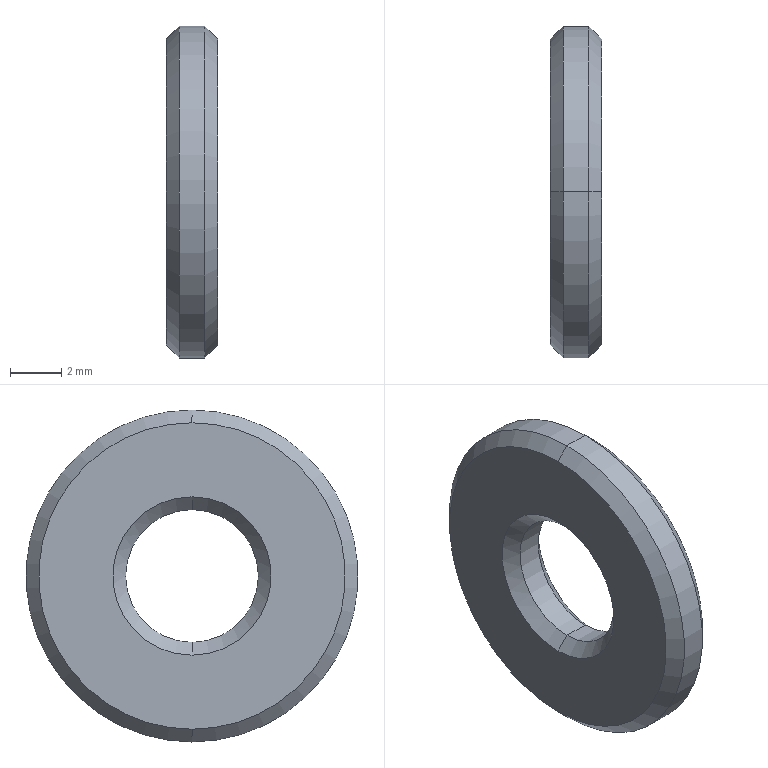Part | STEP file | PN_0018 driven wheel fixing round block_Default | 1 solid | 14 faces | box 2 x 13 x 13 mm | volume 208.696 mm3 | cone 8 | cylinder 4 | plane 2 | commonest cylinder face diameters 5.2 x2 13 x2
STEP:
#1=CARTESIAN_POINT('',(0.,0.,0.));
#2=DIRECTION('',(0.,0.,1.));
#3=DIRECTION('',(1.,0.,0.));
#4=AXIS2_PLACEMENT_3D('',#1,#2,#3);
#5=CARTESIAN_POINT('',(0.5,0.,2.6));
#6=VERTEX_POINT('',#5);
#7=CARTESIAN_POINT('',(0.,0.,3.1));
#8=VERTEX_POINT('',#7);
#9=CARTESIAN_POINT('',(0.,0.,3.1));
#10=DIRECTION('',(-0.7071,0.,0.7071));
#11=VECTOR('',#10,1.);
#12=LINE('',#9,#11);
#13=CARTESIAN_POINT('',(0.,0.,0.));
#14=DIRECTION('',(-1.,0.,0.));
#15=DIRECTION('',(0.,0.,1.));
#16=AXIS2_PLACEMENT_3D('',#13,#14,#15);
#17=CONICAL_SURFACE('',#16,3.1,0.7854);
#18=CARTESIAN_POINT('',(6.283,0.));
#19=DIRECTION('',(0.,1.));
#20=VECTOR('',#19,1.);
#21=LINE('',#18,#20);
#22=(GEOMETRIC_REPRESENTATION_CONTEXT(2)PARAMETRIC_REPRESENTATION_CONTEXT()REPRESENTATION_CONTEXT('',''));
#23=DEFINITIONAL_REPRESENTATION('',(#21),#22);
#24=PCURVE('',#17,#23);
#25=CARTESIAN_POINT('',(0.,0.,0.));
#26=DIRECTION('',(-1.,0.,0.));
#27=DIRECTION('',(0.,0.,1.));
#28=AXIS2_PLACEMENT_3D('',#25,#26,#27);
#29=CONICAL_SURFACE('',#28,3.1,0.7854);
#30=CARTESIAN_POINT('',(0.,0.));
#31=DIRECTION('',(0.,1.));
#32=VECTOR('',#31,1.);
#33=LINE('',#30,#32);
#34=(GEOMETRIC_REPRESENTATION_CONTEXT(2)PARAMETRIC_REPRESENTATION_CONTEXT()REPRESENTATION_CONTEXT('',''));
#35=DEFINITIONAL_REPRESENTATION('',(#33),#34);
#36=PCURVE('',#29,#35);
#37=SURFACE_CURVE('',#12,(#24,#36),.PCURVE_S1.);
#38=EDGE_CURVE('',#6,#8,#37,.T.);
#39=ORIENTED_EDGE('',*,*,#38,.T.);
#40=CARTESIAN_POINT('',(0.,0.,-3.1));
#41=VERTEX_POINT('',#40);
#42=CARTESIAN_POINT('',(0.,0.,0.));
#43=DIRECTION('',(1.,0.,0.));
#44=DIRECTION('',(0.,0.,-1.));
#45=AXIS2_PLACEMENT_3D('',#42,#43,#44);
#46=CIRCLE('',#45,3.1);
#47=CARTESIAN_POINT('',(9.425,0.));
#48=DIRECTION('',(-1.,0.));
#49=VECTOR('',#48,1.);
#50=LINE('',#47,#49);
#51=(GEOMETRIC_REPRESENTATION_CONTEXT(2)PARAMETRIC_REPRESENTATION_CONTEXT()REPRESENTATION_CONTEXT('',''));
#52=DEFINITIONAL_REPRESENTATION('',(#50),#51);
#53=PCURVE('',#17,#52);
#54=CARTESIAN_POINT('',(0.,0.,0.));
#55=DIRECTION('',(1.,0.,0.));
#56=DIRECTION('',(0.,0.,-1.));
#57=AXIS2_PLACEMENT_3D('',#54,#55,#56);
#58=PLANE('',#57);
#59=CARTESIAN_POINT('',(0.,0.));
#60=DIRECTION('',(1.,0.));
#61=AXIS2_PLACEMENT_2D('',#59,#60);
#62=CIRCLE('',#61,3.1);
#63=(GEOMETRIC_REPRESENTATION_CONTEXT(2)PARAMETRIC_REPRESENTATION_CONTEXT()REPRESENTATION_CONTEXT('',''));
#64=DEFINITIONAL_REPRESENTATION('',(#62),#63);
#65=PCURVE('',#58,#64);
#66=SURFACE_CURVE('',#46,(#53,#65),.PCURVE_S1.);
#67=EDGE_CURVE('',#8,#41,#66,.T.);
#68=ORIENTED_EDGE('',*,*,#67,.T.);
#69=CARTESIAN_POINT('',(0.5,0.,-2.6));
#70=VERTEX_POINT('',#69);
#71=CARTESIAN_POINT('',(0.,0.,-3.1));
#72=DIRECTION('',(-0.7071,0.,-0.7071));
#73=VECTOR('',#72,1.);
#74=LINE('',#71,#73);
#75=CARTESIAN_POINT('',(3.142,0.));
#76=DIRECTION('',(0.,1.));
#77=VECTOR('',#76,1.);
#78=LINE('',#75,#77);
#79=(GEOMETRIC_REPRESENTATION_CONTEXT(2)PARAMETRIC_REPRESENTATION_CONTEXT()REPRESENTATION_CONTEXT('',''));
#80=DEFINITIONAL_REPRESENTATION('',(#78),#79);
#81=PCURVE('',#17,#80);
#82=CARTESIAN_POINT('',(3.142,0.));
#83=DIRECTION('',(0.,1.));
#84=VECTOR('',#83,1.);
#85=LINE('',#82,#84);
#86=(GEOMETRIC_REPRESENTATION_CONTEXT(2)PARAMETRIC_REPRESENTATION_CONTEXT()REPRESENTATION_CONTEXT('',''));
#87=DEFINITIONAL_REPRESENTATION('',(#85),#86);
#88=PCURVE('',#29,#87);
#89=SURFACE_CURVE('',#74,(#81,#88),.PCURVE_S1.);
#90=EDGE_CURVE('',#70,#41,#89,.T.);
#91=ORIENTED_EDGE('',*,*,#90,.F.);
#92=CARTESIAN_POINT('',(0.5,0.,0.));
#93=DIRECTION('',(-1.,0.,0.));
#94=DIRECTION('',(0.,0.,-1.));
#95=AXIS2_PLACEMENT_3D('',#92,#93,#94);
#96=CIRCLE('',#95,2.6);
#97=CARTESIAN_POINT('',(3.142,-0.5));
#98=DIRECTION('',(1.,0.));
#99=VECTOR('',#98,1.);
#100=LINE('',#97,#99);
#101=(GEOMETRIC_REPRESENTATION_CONTEXT(2)PARAMETRIC_REPRESENTATION_CONTEXT()REPRESENTATION_CONTEXT('',''));
#102=DEFINITIONAL_REPRESENTATION('',(#100),#101);
#103=PCURVE('',#17,#102);
#104=CARTESIAN_POINT('',(2.,0.,0.));
#105=DIRECTION('',(-1.,0.,0.));
#106=DIRECTION('',(0.,0.,1.));
#107=AXIS2_PLACEMENT_3D('',#104,#105,#106);
#108=CYLINDRICAL_SURFACE('',#107,2.6);
#109=CARTESIAN_POINT('',(3.142,1.5));
#110=DIRECTION('',(1.,0.));
#111=VECTOR('',#110,1.);
#112=LINE('',#109,#111);
#113=(GEOMETRIC_REPRESENTATION_CONTEXT(2)PARAMETRIC_REPRESENTATION_CONTEXT()REPRESENTATION_CONTEXT('',''));
#114=DEFINITIONAL_REPRESENTATION('',(#112),#113);
#115=PCURVE('',#108,#114);
#116=SURFACE_CURVE('',#96,(#103,#115),.PCURVE_S1.);
#117=EDGE_CURVE('',#70,#6,#116,.T.);
#118=ORIENTED_EDGE('',*,*,#117,.T.);
#119=EDGE_LOOP('',(#39,#68,#91,#118));
#120=FACE_BOUND('',#119,.F.);
#121=ADVANCED_FACE('',(#120),#17,.F.);
#122=CARTESIAN_POINT('',(1.5,0.,-2.6));
#123=VERTEX_POINT('',#122);
#124=CARTESIAN_POINT('',(2.,0.,-3.1));
#125=VERTEX_POINT('',#124);
#126=CARTESIAN_POINT('',(1.5,0.,-2.6));
#127=DIRECTION('',(0.7071,0.,-0.7071));
#128=VECTOR('',#127,1.);
#129=LINE('',#126,#128);
#130=CARTESIAN_POINT('',(1.5,0.,0.));
#131=DIRECTION('',(1.,0.,0.));
#132=DIRECTION('',(0.,0.,-1.));
#133=AXIS2_PLACEMENT_3D('',#130,#131,#132);
#134=CONICAL_SURFACE('',#133,2.6,0.7854);
#135=CARTESIAN_POINT('',(6.283,0.));
#136=DIRECTION('',(0.,1.));
#137=VECTOR('',#136,1.);
#138=LINE('',#135,#137);
#139=(GEOMETRIC_REPRESENTATION_CONTEXT(2)PARAMETRIC_REPRESENTATION_CONTEXT()REPRESENTATION_CONTEXT('',''));
#140=DEFINITIONAL_REPRESENTATION('',(#138),#139);
#141=PCURVE('',#134,#140);
#142=CARTESIAN_POINT('',(1.5,0.,0.));
#143=DIRECTION('',(1.,0.,0.));
#144=DIRECTION('',(0.,0.,-1.));
#145=AXIS2_PLACEMENT_3D('',#142,#143,#144);
#146=CONICAL_SURFACE('',#145,2.6,0.7854);
#147=CARTESIAN_POINT('',(0.,0.));
#148=DIRECTION('',(0.,1.));
#149=VECTOR('',#148,1.);
#150=LINE('',#147,#149);
#151=(GEOMETRIC_REPRESENTATION_CONTEXT(2)PARAMETRIC_REPRESENTATION_CONTEXT()REPRESENTATION_CONTEXT('',''));
#152=DEFINITIONAL_REPRESENTATION('',(#150),#151);
#153=PCURVE('',#146,#152);
#154=SURFACE_CURVE('',#129,(#141,#153),.PCURVE_S1.);
#155=EDGE_CURVE('',#123,#125,#154,.T.);
#156=ORIENTED_EDGE('',*,*,#155,.T.);
#157=CARTESIAN_POINT('',(2.,0.,3.1));
#158=VERTEX_POINT('',#157);
#159=CARTESIAN_POINT('',(2.,0.,0.));
#160=DIRECTION('',(-1.,0.,0.));
#161=DIRECTION('',(0.,0.,-1.));
#162=AXIS2_PLACEMENT_3D('',#159,#160,#161);
#163=CIRCLE('',#162,3.1);
#164=CARTESIAN_POINT('',(6.283,0.5));
#165=DIRECTION('',(-1.,0.));
#166=VECTOR('',#165,1.);
#167=LINE('',#164,#166);
#168=(GEOMETRIC_REPRESENTATION_CONTEXT(2)PARAMETRIC_REPRESENTATION_CONTEXT()REPRESENTATION_CONTEXT('',''));
#169=DEFINITIONAL_REPRESENTATION('',(#167),#168);
#170=PCURVE('',#134,#169);
#171=CARTESIAN_POINT('',(2.,0.,0.));
#172=DIRECTION('',(1.,0.,0.));
#173=DIRECTION('',(0.,0.,-1.));
#174=AXIS2_PLACEMENT_3D('',#171,#172,#173);
#175=PLANE('',#174);
#176=CARTESIAN_POINT('',(3.1,0.));
#177=CARTESIAN_POINT('',(3.1,-5.369));
#178=CARTESIAN_POINT('',(-1.55,-2.685));
#179=CARTESIAN_POINT('',(-6.2,0.));
#180=CARTESIAN_POINT('',(-1.55,2.685));
#181=CARTESIAN_POINT('',(3.1,5.369));
#182=CARTESIAN_POINT('',(3.1,0.));
#183=(BOUNDED_CURVE()B_SPLINE_CURVE(2,(#176,#177,#178,#179,#180,#181,#182),.UNSPECIFIED.,.T.,.F.)B_SPLINE_CURVE_WITH_KNOTS((1,2,2,2,2,1),(-2.094,0.,2.094,4.189,6.283,8.378),.UNSPECIFIED.)CURVE()GEOMETRIC_REPRESENTATION_ITEM()RATIONAL_B_SPLINE_CURVE((1.,0.5,1.,0.5,1.,0.5,1.))REPRESENTATION_ITEM(''));
#184=(GEOMETRIC_REPRESENTATION_CONTEXT(2)PARAMETRIC_REPRESENTATION_CONTEXT()REPRESENTATION_CONTEXT('',''));
#185=DEFINITIONAL_REPRESENTATION('',(#183),#184);
#186=PCURVE('',#175,#185);
#187=SURFACE_CURVE('',#163,(#170,#186),.PCURVE_S1.);
#188=EDGE_CURVE('',#125,#158,#187,.T.);
#189=ORIENTED_EDGE('',*,*,#188,.T.);
#190=CARTESIAN_POINT('',(1.5,0.,2.6));
#191=VERTEX_POINT('',#190);
#192=CARTESIAN_POINT('',(1.5,0.,2.6));
#193=DIRECTION('',(0.7071,0.,0.7071));
#194=VECTOR('',#193,1.);
#195=LINE('',#192,#194);
#196=CARTESIAN_POINT('',(3.142,0.));
#197=DIRECTION('',(0.,1.));
#198=VECTOR('',#197,1.);
#199=LINE('',#196,#198);
#200=(GEOMETRIC_REPRESENTATION_CONTEXT(2)PARAMETRIC_REPRESENTATION_CONTEXT()REPRESENTATION_CONTEXT('',''));
#201=DEFINITIONAL_REPRESENTATION('',(#199),#200);
#202=PCURVE('',#134,#201);
#203=CARTESIAN_POINT('',(3.142,0.));
#204=DIRECTION('',(0.,1.));
#205=VECTOR('',#204,1.);
#206=LINE('',#203,#205);
#207=(GEOMETRIC_REPRESENTATION_CONTEXT(2)PARAMETRIC_REPRESENTATION_CONTEXT()REPRESENTATION_CONTEXT('',''));
#208=DEFINITIONAL_REPRESENTATION('',(#206),#207);
#209=PCURVE('',#146,#208);
#210=SURFACE_CURVE('',#195,(#202,#209),.PCURVE_S1.);
#211=EDGE_CURVE('',#191,#158,#210,.T.);
#212=ORIENTED_EDGE('',*,*,#211,.F.);
#213=CARTESIAN_POINT('',(1.5,0.,0.));
#214=DIRECTION('',(1.,0.,0.));
#215=DIRECTION('',(0.,0.,-1.));
#216=AXIS2_PLACEMENT_3D('',#213,#214,#215);
#217=CIRCLE('',#216,2.6);
#218=CARTESIAN_POINT('',(0.,0.));
#219=DIRECTION('',(1.,0.));
#220=VECTOR('',#219,1.);
#221=LINE('',#218,#220);
#222=(GEOMETRIC_REPRESENTATION_CONTEXT(2)PARAMETRIC_REPRESENTATION_CONTEXT()REPRESENTATION_CONTEXT('',''));
#223=DEFINITIONAL_REPRESENTATION('',(#221),#222);
#224=PCURVE('',#134,#223);
#225=CARTESIAN_POINT('',(9.425,0.5));
#226=DIRECTION('',(-1.,0.));
#227=VECTOR('',#226,1.);
#228=LINE('',#225,#227);
#229=(GEOMETRIC_REPRESENTATION_CONTEXT(2)PARAMETRIC_REPRESENTATION_CONTEXT()REPRESENTATION_CONTEXT('',''));
#230=DEFINITIONAL_REPRESENTATION('',(#228),#229);
#231=PCURVE('',#108,#230);
#232=SURFACE_CURVE('',#217,(#224,#231),.PCURVE_S1.);
#233=EDGE_CURVE('',#191,#123,#232,.T.);
#234=ORIENTED_EDGE('',*,*,#233,.T.);
#235=EDGE_LOOP('',(#156,#189,#212,#234));
#236=FACE_BOUND('',#235,.F.);
#237=ADVANCED_FACE('',(#236),#134,.F.);
#238=CARTESIAN_POINT('',(0.,0.,6.));
#239=VERTEX_POINT('',#238);
#240=CARTESIAN_POINT('',(0.,0.,-6.));
#241=VERTEX_POINT('',#240);
#242=CARTESIAN_POINT('',(0.,0.,0.));
#243=DIRECTION('',(-1.,0.,0.));
#244=DIRECTION('',(0.,0.,-1.));
#245=AXIS2_PLACEMENT_3D('',#242,#243,#244);
#246=CIRCLE('',#245,6.);
#247=CARTESIAN_POINT('',(0.5,0.,0.));
#248=DIRECTION('',(1.,0.,0.));
#249=DIRECTION('',(0.,0.,-1.));
#250=AXIS2_PLACEMENT_3D('',#247,#248,#249);
#251=CONICAL_SURFACE('',#250,6.5,0.7854);
#252=CARTESIAN_POINT('',(6.283,-0.5));
#253=DIRECTION('',(-1.,0.));
#254=VECTOR('',#253,1.);
#255=LINE('',#252,#254);
#256=(GEOMETRIC_REPRESENTATION_CONTEXT(2)PARAMETRIC_REPRESENTATION_CONTEXT()REPRESENTATION_CONTEXT('',''));
#257=DEFINITIONAL_REPRESENTATION('',(#255),#256);
#258=PCURVE('',#251,#257);
#259=CARTESIAN_POINT('',(6.,0.));
#260=CARTESIAN_POINT('',(6.,-10.392));
#261=CARTESIAN_POINT('',(-3.,-5.196));
#262=CARTESIAN_POINT('',(-12.,0.));
#263=CARTESIAN_POINT('',(-3.,5.196));
#264=CARTESIAN_POINT('',(6.,10.392));
#265=CARTESIAN_POINT('',(6.,0.));
#266=(BOUNDED_CURVE()B_SPLINE_CURVE(2,(#259,#260,#261,#262,#263,#264,#265),.UNSPECIFIED.,.T.,.F.)B_SPLINE_CURVE_WITH_KNOTS((1,2,2,2,2,1),(-2.094,0.,2.094,4.189,6.283,8.378),.UNSPECIFIED.)CURVE()GEOMETRIC_REPRESENTATION_ITEM()RATIONAL_B_SPLINE_CURVE((1.,0.5,1.,0.5,1.,0.5,1.))REPRESENTATION_ITEM(''));
#267=(GEOMETRIC_REPRESENTATION_CONTEXT(2)PARAMETRIC_REPRESENTATION_CONTEXT()REPRESENTATION_CONTEXT('',''));
#268=DEFINITIONAL_REPRESENTATION('',(#266),#267);
#269=PCURVE('',#58,#268);
#270=SURFACE_CURVE('',#246,(#258,#269),.PCURVE_S1.);
#271=EDGE_CURVE('',#239,#241,#270,.T.);
#272=ORIENTED_EDGE('',*,*,#271,.F.);
#273=CARTESIAN_POINT('',(0.5,0.,6.5));
#274=VERTEX_POINT('',#273);
#275=CARTESIAN_POINT('',(0.5,0.,6.5));
#276=DIRECTION('',(0.7071,0.,0.7071));
#277=VECTOR('',#276,1.);
#278=LINE('',#275,#277);
#279=CARTESIAN_POINT('',(3.142,0.));
#280=DIRECTION('',(0.,1.));
#281=VECTOR('',#280,1.);
#282=LINE('',#279,#281);
#283=(GEOMETRIC_REPRESENTATION_CONTEXT(2)PARAMETRIC_REPRESENTATION_CONTEXT()REPRESENTATION_CONTEXT('',''));
#284=DEFINITIONAL_REPRESENTATION('',(#282),#283);
#285=PCURVE('',#251,#284);
#286=CARTESIAN_POINT('',(0.5,0.,0.));
#287=DIRECTION('',(1.,0.,0.));
#288=DIRECTION('',(0.,0.,-1.));
#289=AXIS2_PLACEMENT_3D('',#286,#287,#288);
#290=CONICAL_SURFACE('',#289,6.5,0.7854);
#291=CARTESIAN_POINT('',(3.142,0.));
#292=DIRECTION('',(0.,1.));
#293=VECTOR('',#292,1.);
#294=LINE('',#291,#293);
#295=(GEOMETRIC_REPRESENTATION_CONTEXT(2)PARAMETRIC_REPRESENTATION_CONTEXT()REPRESENTATION_CONTEXT('',''));
#296=DEFINITIONAL_REPRESENTATION('',(#294),#295);
#297=PCURVE('',#290,#296);
#298=SURFACE_CURVE('',#278,(#285,#297),.PCURVE_S1.);
#299=EDGE_CURVE('',#239,#274,#298,.T.);
#300=ORIENTED_EDGE('',*,*,#299,.T.);
#301=CARTESIAN_POINT('',(0.5,0.,-6.5));
#302=VERTEX_POINT('',#301);
#303=CARTESIAN_POINT('',(0.5,0.,0.));
#304=DIRECTION('',(1.,0.,0.));
#305=DIRECTION('',(0.,0.,-1.));
#306=AXIS2_PLACEMENT_3D('',#303,#304,#305);
#307=CIRCLE('',#306,6.5);
#308=CARTESIAN_POINT('',(0.,0.));
#309=DIRECTION('',(1.,0.));
#310=VECTOR('',#309,1.);
#311=LINE('',#308,#310);
#312=(GEOMETRIC_REPRESENTATION_CONTEXT(2)PARAMETRIC_REPRESENTATION_CONTEXT()REPRESENTATION_CONTEXT('',''));
#313=DEFINITIONAL_REPRESENTATION('',(#311),#312);
#314=PCURVE('',#251,#313);
#315=CARTESIAN_POINT('',(2.,0.,0.));
#316=DIRECTION('',(-1.,0.,0.));
#317=DIRECTION('',(0.,0.,1.));
#318=AXIS2_PLACEMENT_3D('',#315,#316,#317);
#319=CYLINDRICAL_SURFACE('',#318,6.5);
#320=CARTESIAN_POINT('',(3.142,1.5));
#321=DIRECTION('',(-1.,0.));
#322=VECTOR('',#321,1.);
#323=LINE('',#320,#322);
#324=(GEOMETRIC_REPRESENTATION_CONTEXT(2)PARAMETRIC_REPRESENTATION_CONTEXT()REPRESENTATION_CONTEXT('',''));
#325=DEFINITIONAL_REPRESENTATION('',(#323),#324);
#326=PCURVE('',#319,#325);
#327=SURFACE_CURVE('',#307,(#314,#326),.PCURVE_S1.);
#328=EDGE_CURVE('',#302,#274,#327,.T.);
#329=ORIENTED_EDGE('',*,*,#328,.F.);
#330=CARTESIAN_POINT('',(0.5,0.,-6.5));
#331=DIRECTION('',(0.7071,0.,-0.7071));
#332=VECTOR('',#331,1.);
#333=LINE('',#330,#332);
#334=CARTESIAN_POINT('',(0.,0.));
#335=DIRECTION('',(0.,1.));
#336=VECTOR('',#335,1.);
#337=LINE('',#334,#336);
#338=(GEOMETRIC_REPRESENTATION_CONTEXT(2)PARAMETRIC_REPRESENTATION_CONTEXT()REPRESENTATION_CONTEXT('',''));
#339=DEFINITIONAL_REPRESENTATION('',(#337),#338);
#340=PCURVE('',#251,#339);
#341=CARTESIAN_POINT('',(6.283,0.));
#342=DIRECTION('',(0.,1.));
#343=VECTOR('',#342,1.);
#344=LINE('',#341,#343);
#345=(GEOMETRIC_REPRESENTATION_CONTEXT(2)PARAMETRIC_REPRESENTATION_CONTEXT()REPRESENTATION_CONTEXT('',''));
#346=DEFINITIONAL_REPRESENTATION('',(#344),#345);
#347=PCURVE('',#290,#346);
#348=SURFACE_CURVE('',#333,(#340,#347),.PCURVE_S1.);
#349=EDGE_CURVE('',#241,#302,#348,.T.);
#350=ORIENTED_EDGE('',*,*,#349,.F.);
#351=EDGE_LOOP('',(#272,#300,#329,#350));
#352=FACE_BOUND('',#351,.T.);
#353=ADVANCED_FACE('',(#352),#251,.T.);
#354=CARTESIAN_POINT('',(2.,0.,-6.));
#355=VERTEX_POINT('',#354);
#356=CARTESIAN_POINT('',(2.,0.,6.));
#357=VERTEX_POINT('',#356);
#358=CARTESIAN_POINT('',(2.,0.,0.));
#359=DIRECTION('',(1.,0.,0.));
#360=DIRECTION('',(0.,0.,-1.));
#361=AXIS2_PLACEMENT_3D('',#358,#359,#360);
#362=CIRCLE('',#361,6.);
#363=CARTESIAN_POINT('',(2.,0.,0.));
#364=DIRECTION('',(-1.,0.,0.));
#365=DIRECTION('',(0.,0.,1.));
#366=AXIS2_PLACEMENT_3D('',#363,#364,#365);
#367=CONICAL_SURFACE('',#366,6.,0.7854);
#368=CARTESIAN_POINT('',(3.142,0.));
#369=DIRECTION('',(-1.,0.));
#370=VECTOR('',#369,1.);
#371=LINE('',#368,#370);
#372=(GEOMETRIC_REPRESENTATION_CONTEXT(2)PARAMETRIC_REPRESENTATION_CONTEXT()REPRESENTATION_CONTEXT('',''));
#373=DEFINITIONAL_REPRESENTATION('',(#371),#372);
#374=PCURVE('',#367,#373);
#375=CARTESIAN_POINT('',(0.,0.));
#376=DIRECTION('',(1.,0.));
#377=AXIS2_PLACEMENT_2D('',#375,#376);
#378=CIRCLE('',#377,6.);
#379=(GEOMETRIC_REPRESENTATION_CONTEXT(2)PARAMETRIC_REPRESENTATION_CONTEXT()REPRESENTATION_CONTEXT('',''));
#380=DEFINITIONAL_REPRESENTATION('',(#378),#379);
#381=PCURVE('',#175,#380);
#382=SURFACE_CURVE('',#362,(#374,#381),.PCURVE_S1.);
#383=EDGE_CURVE('',#355,#357,#382,.T.);
#384=ORIENTED_EDGE('',*,*,#383,.F.);
#385=CARTESIAN_POINT('',(1.5,0.,-6.5));
#386=VERTEX_POINT('',#385);
#387=CARTESIAN_POINT('',(2.,0.,-6.));
#388=DIRECTION('',(-0.7071,0.,-0.7071));
#389=VECTOR('',#388,1.);
#390=LINE('',#387,#389);
#391=CARTESIAN_POINT('',(3.142,0.));
#392=DIRECTION('',(0.,1.));
#393=VECTOR('',#392,1.);
#394=LINE('',#391,#393);
#395=(GEOMETRIC_REPRESENTATION_CONTEXT(2)PARAMETRIC_REPRESENTATION_CONTEXT()REPRESENTATION_CONTEXT('',''));
#396=DEFINITIONAL_REPRESENTATION('',(#394),#395);
#397=PCURVE('',#367,#396);
#398=CARTESIAN_POINT('',(2.,0.,0.));
#399=DIRECTION('',(-1.,0.,0.));
#400=DIRECTION('',(0.,0.,1.));
#401=AXIS2_PLACEMENT_3D('',#398,#399,#400);
#402=CONICAL_SURFACE('',#401,6.,0.7854);
#403=CARTESIAN_POINT('',(3.142,0.));
#404=DIRECTION('',(0.,1.));
#405=VECTOR('',#404,1.);
#406=LINE('',#403,#405);
#407=(GEOMETRIC_REPRESENTATION_CONTEXT(2)PARAMETRIC_REPRESENTATION_CONTEXT()REPRESENTATION_CONTEXT('',''));
#408=DEFINITIONAL_REPRESENTATION('',(#406),#407);
#409=PCURVE('',#402,#408);
#410=SURFACE_CURVE('',#390,(#397,#409),.PCURVE_S1.);
#411=EDGE_CURVE('',#355,#386,#410,.T.);
#412=ORIENTED_EDGE('',*,*,#411,.T.);
#413=CARTESIAN_POINT('',(1.5,0.,6.5));
#414=VERTEX_POINT('',#413);
#415=CARTESIAN_POINT('',(1.5,0.,0.));
#416=DIRECTION('',(-1.,0.,0.));
#417=DIRECTION('',(0.,0.,-1.));
#418=AXIS2_PLACEMENT_3D('',#415,#416,#417);
#419=CIRCLE('',#418,6.5);
#420=CARTESIAN_POINT('',(-3.142,0.5));
#421=DIRECTION('',(1.,0.));
#422=VECTOR('',#421,1.);
#423=LINE('',#420,#422);
#424=(GEOMETRIC_REPRESENTATION_CONTEXT(2)PARAMETRIC_REPRESENTATION_CONTEXT()REPRESENTATION_CONTEXT('',''));
#425=DEFINITIONAL_REPRESENTATION('',(#423),#424);
#426=PCURVE('',#367,#425);
#427=CARTESIAN_POINT('',(-3.142,0.5));
#428=DIRECTION('',(1.,0.));
#429=VECTOR('',#428,1.);
#430=LINE('',#427,#429);
#431=(GEOMETRIC_REPRESENTATION_CONTEXT(2)PARAMETRIC_REPRESENTATION_CONTEXT()REPRESENTATION_CONTEXT('',''));
#432=DEFINITIONAL_REPRESENTATION('',(#430),#431);
#433=PCURVE('',#319,#432);
#434=SURFACE_CURVE('',#419,(#426,#433),.PCURVE_S1.);
#435=EDGE_CURVE('',#414,#386,#434,.T.);
#436=ORIENTED_EDGE('',*,*,#435,.F.);
#437=CARTESIAN_POINT('',(2.,0.,6.));
#438=DIRECTION('',(-0.7071,0.,0.7071));
#439=VECTOR('',#438,1.);
#440=LINE('',#437,#439);
#441=CARTESIAN_POINT('',(0.,0.));
#442=DIRECTION('',(0.,1.));
#443=VECTOR('',#442,1.);
#444=LINE('',#441,#443);
#445=(GEOMETRIC_REPRESENTATION_CONTEXT(2)PARAMETRIC_REPRESENTATION_CONTEXT()REPRESENTATION_CONTEXT('',''));
#446=DEFINITIONAL_REPRESENTATION('',(#444),#445);
#447=PCURVE('',#367,#446);
#448=CARTESIAN_POINT('',(6.283,0.));
#449=DIRECTION('',(0.,1.));
#450=VECTOR('',#449,1.);
#451=LINE('',#448,#450);
#452=(GEOMETRIC_REPRESENTATION_CONTEXT(2)PARAMETRIC_REPRESENTATION_CONTEXT()REPRESENTATION_CONTEXT('',''));
#453=DEFINITIONAL_REPRESENTATION('',(#451),#452);
#454=PCURVE('',#402,#453);
#455=SURFACE_CURVE('',#440,(#447,#454),.PCURVE_S1.);
#456=EDGE_CURVE('',#357,#414,#455,.T.);
#457=ORIENTED_EDGE('',*,*,#456,.F.);
#458=EDGE_LOOP('',(#384,#412,#436,#457));
#459=FACE_BOUND('',#458,.T.);
#460=ADVANCED_FACE('',(#459),#367,.T.);
#461=CARTESIAN_POINT('',(2.,0.,2.6));
#462=DIRECTION('',(-1.,0.,0.));
#463=VECTOR('',#462,1.);
#464=LINE('',#461,#463);
#465=CARTESIAN_POINT('',(6.283,0.));
#466=DIRECTION('',(0.,1.));
#467=VECTOR('',#466,1.);
#468=LINE('',#465,#467);
#469=(GEOMETRIC_REPRESENTATION_CONTEXT(2)PARAMETRIC_REPRESENTATION_CONTEXT()REPRESENTATION_CONTEXT('',''));
#470=DEFINITIONAL_REPRESENTATION('',(#468),#469);
#471=PCURVE('',#108,#470);
#472=CARTESIAN_POINT('',(2.,0.,0.));
#473=DIRECTION('',(-1.,0.,0.));
#474=DIRECTION('',(0.,0.,1.));
#475=AXIS2_PLACEMENT_3D('',#472,#473,#474);
#476=CYLINDRICAL_SURFACE('',#475,2.6);
#477=CARTESIAN_POINT('',(0.,0.));
#478=DIRECTION('',(0.,1.));
#479=VECTOR('',#478,1.);
#480=LINE('',#477,#479);
#481=(GEOMETRIC_REPRESENTATION_CONTEXT(2)PARAMETRIC_REPRESENTATION_CONTEXT()REPRESENTATION_CONTEXT('',''));
#482=DEFINITIONAL_REPRESENTATION('',(#480),#481);
#483=PCURVE('',#476,#482);
#484=SURFACE_CURVE('',#464,(#471,#483),.PCURVE_S1.);
#485=EDGE_CURVE('',#191,#6,#484,.T.);
#486=ORIENTED_EDGE('',*,*,#485,.T.);
#487=ORIENTED_EDGE('',*,*,#117,.F.);
#488=CARTESIAN_POINT('',(2.,0.,-2.6));
#489=DIRECTION('',(-1.,0.,0.));
#490=VECTOR('',#489,1.);
#491=LINE('',#488,#490);
#492=CARTESIAN_POINT('',(3.142,0.));
#493=DIRECTION('',(0.,1.));
#494=VECTOR('',#493,1.);
#495=LINE('',#492,#494);
#496=(GEOMETRIC_REPRESENTATION_CONTEXT(2)PARAMETRIC_REPRESENTATION_CONTEXT()REPRESENTATION_CONTEXT('',''));
#497=DEFINITIONAL_REPRESENTATION('',(#495),#496);
#498=PCURVE('',#108,#497);
#499=CARTESIAN_POINT('',(3.142,0.));
#500=DIRECTION('',(0.,1.));
#501=VECTOR('',#500,1.);
#502=LINE('',#499,#501);
#503=(GEOMETRIC_REPRESENTATION_CONTEXT(2)PARAMETRIC_REPRESENTATION_CONTEXT()REPRESENTATION_CONTEXT('',''));
#504=DEFINITIONAL_REPRESENTATION('',(#502),#503);
#505=PCURVE('',#476,#504);
#506=SURFACE_CURVE('',#491,(#498,#505),.PCURVE_S1.);
#507=EDGE_CURVE('',#123,#70,#506,.T.);
#508=ORIENTED_EDGE('',*,*,#507,.F.);
#509=ORIENTED_EDGE('',*,*,#233,.F.);
#510=EDGE_LOOP('',(#486,#487,#508,#509));
#511=FACE_BOUND('',#510,.F.);
#512=ADVANCED_FACE('',(#511),#108,.F.);
#513=ORIENTED_EDGE('',*,*,#435,.T.);
#514=CARTESIAN_POINT('',(2.,0.,-6.5));
#515=DIRECTION('',(-1.,0.,0.));
#516=VECTOR('',#515,1.);
#517=LINE('',#514,#516);
#518=CARTESIAN_POINT('',(3.142,0.));
#519=DIRECTION('',(0.,1.));
#520=VECTOR('',#519,1.);
#521=LINE('',#518,#520);
#522=(GEOMETRIC_REPRESENTATION_CONTEXT(2)PARAMETRIC_REPRESENTATION_CONTEXT()REPRESENTATION_CONTEXT('',''));
#523=DEFINITIONAL_REPRESENTATION('',(#521),#522);
#524=PCURVE('',#319,#523);
#525=CARTESIAN_POINT('',(2.,0.,0.));
#526=DIRECTION('',(-1.,0.,0.));
#527=DIRECTION('',(0.,0.,1.));
#528=AXIS2_PLACEMENT_3D('',#525,#526,#527);
#529=CYLINDRICAL_SURFACE('',#528,6.5);
#530=CARTESIAN_POINT('',(3.142,0.));
#531=DIRECTION('',(0.,1.));
#532=VECTOR('',#531,1.);
#533=LINE('',#530,#532);
#534=(GEOMETRIC_REPRESENTATION_CONTEXT(2)PARAMETRIC_REPRESENTATION_CONTEXT()REPRESENTATION_CONTEXT('',''));
#535=DEFINITIONAL_REPRESENTATION('',(#533),#534);
#536=PCURVE('',#529,#535);
#537=SURFACE_CURVE('',#517,(#524,#536),.PCURVE_S1.);
#538=EDGE_CURVE('',#386,#302,#537,.T.);
#539=ORIENTED_EDGE('',*,*,#538,.T.);
#540=ORIENTED_EDGE('',*,*,#328,.T.);
#541=CARTESIAN_POINT('',(2.,0.,6.5));
#542=DIRECTION('',(-1.,0.,0.));
#543=VECTOR('',#542,1.);
#544=LINE('',#541,#543);
#545=CARTESIAN_POINT('',(0.,0.));
#546=DIRECTION('',(0.,1.));
#547=VECTOR('',#546,1.);
#548=LINE('',#545,#547);
#549=(GEOMETRIC_REPRESENTATION_CONTEXT(2)PARAMETRIC_REPRESENTATION_CONTEXT()REPRESENTATION_CONTEXT('',''));
#550=DEFINITIONAL_REPRESENTATION('',(#548),#549);
#551=PCURVE('',#319,#550);
#552=CARTESIAN_POINT('',(6.283,0.));
#553=DIRECTION('',(0.,1.));
#554=VECTOR('',#553,1.);
#555=LINE('',#552,#554);
#556=(GEOMETRIC_REPRESENTATION_CONTEXT(2)PARAMETRIC_REPRESENTATION_CONTEXT()REPRESENTATION_CONTEXT('',''));
#557=DEFINITIONAL_REPRESENTATION('',(#555),#556);
#558=PCURVE('',#529,#557);
#559=SURFACE_CURVE('',#544,(#551,#558),.PCURVE_S1.);
#560=EDGE_CURVE('',#414,#274,#559,.T.);
#561=ORIENTED_EDGE('',*,*,#560,.F.);
#562=EDGE_LOOP('',(#513,#539,#540,#561));
#563=FACE_BOUND('',#562,.T.);
#564=ADVANCED_FACE('',(#563),#319,.T.);
#565=CARTESIAN_POINT('',(2.,0.,0.));
#566=DIRECTION('',(1.,0.,0.));
#567=DIRECTION('',(0.,0.,-1.));
#568=AXIS2_PLACEMENT_3D('',#565,#566,#567);
#569=CIRCLE('',#568,6.);
#570=CARTESIAN_POINT('',(0.,0.));
#571=DIRECTION('',(1.,0.));
#572=AXIS2_PLACEMENT_2D('',#570,#571);
#573=CIRCLE('',#572,6.);
#574=(GEOMETRIC_REPRESENTATION_CONTEXT(2)PARAMETRIC_REPRESENTATION_CONTEXT()REPRESENTATION_CONTEXT('',''));
#575=DEFINITIONAL_REPRESENTATION('',(#573),#574);
#576=PCURVE('',#175,#575);
#577=CARTESIAN_POINT('',(9.425,0.));
#578=DIRECTION('',(-1.,0.));
#579=VECTOR('',#578,1.);
#580=LINE('',#577,#579);
#581=(GEOMETRIC_REPRESENTATION_CONTEXT(2)PARAMETRIC_REPRESENTATION_CONTEXT()REPRESENTATION_CONTEXT('',''));
#582=DEFINITIONAL_REPRESENTATION('',(#580),#581);
#583=PCURVE('',#402,#582);
#584=SURFACE_CURVE('',#569,(#576,#583),.PCURVE_S1.);
#585=EDGE_CURVE('',#357,#355,#584,.T.);
#586=ORIENTED_EDGE('',*,*,#585,.T.);
#587=ORIENTED_EDGE('',*,*,#383,.T.);
#588=EDGE_LOOP('',(#586,#587));
#589=FACE_BOUND('',#588,.T.);
#590=ORIENTED_EDGE('',*,*,#188,.T.);
#591=CARTESIAN_POINT('',(2.,0.,0.));
#592=DIRECTION('',(-1.,0.,0.));
#593=DIRECTION('',(0.,0.,-1.));
#594=AXIS2_PLACEMENT_3D('',#591,#592,#593);
#595=CIRCLE('',#594,3.1);
#596=CARTESIAN_POINT('',(3.1,0.));
#597=CARTESIAN_POINT('',(3.1,-5.369));
#598=CARTESIAN_POINT('',(-1.55,-2.685));
#599=CARTESIAN_POINT('',(-6.2,0.));
#600=CARTESIAN_POINT('',(-1.55,2.685));
#601=CARTESIAN_POINT('',(3.1,5.369));
#602=CARTESIAN_POINT('',(3.1,0.));
#603=(BOUNDED_CURVE()B_SPLINE_CURVE(2,(#596,#597,#598,#599,#600,#601,#602),.UNSPECIFIED.,.T.,.F.)B_SPLINE_CURVE_WITH_KNOTS((1,2,2,2,2,1),(-2.094,0.,2.094,4.189,6.283,8.378),.UNSPECIFIED.)CURVE()GEOMETRIC_REPRESENTATION_ITEM()RATIONAL_B_SPLINE_CURVE((1.,0.5,1.,0.5,1.,0.5,1.))REPRESENTATION_ITEM(''));
#604=(GEOMETRIC_REPRESENTATION_CONTEXT(2)PARAMETRIC_REPRESENTATION_CONTEXT()REPRESENTATION_CONTEXT('',''));
#605=DEFINITIONAL_REPRESENTATION('',(#603),#604);
#606=PCURVE('',#175,#605);
#607=CARTESIAN_POINT('',(6.283,0.5));
#608=DIRECTION('',(-1.,0.));
#609=VECTOR('',#608,1.);
#610=LINE('',#607,#609);
#611=(GEOMETRIC_REPRESENTATION_CONTEXT(2)PARAMETRIC_REPRESENTATION_CONTEXT()REPRESENTATION_CONTEXT('',''));
#612=DEFINITIONAL_REPRESENTATION('',(#610),#611);
#613=PCURVE('',#146,#612);
#614=SURFACE_CURVE('',#595,(#606,#613),.PCURVE_S1.);
#615=EDGE_CURVE('',#158,#125,#614,.T.);
#616=ORIENTED_EDGE('',*,*,#615,.T.);
#617=EDGE_LOOP('',(#590,#616));
#618=FACE_BOUND('',#617,.T.);
#619=ADVANCED_FACE('',(#589,#618),#175,.T.);
#620=CARTESIAN_POINT('',(0.,0.,0.));
#621=DIRECTION('',(-1.,0.,0.));
#622=DIRECTION('',(0.,0.,-1.));
#623=AXIS2_PLACEMENT_3D('',#620,#621,#622);
#624=CIRCLE('',#623,6.);
#625=CARTESIAN_POINT('',(6.,0.));
#626=CARTESIAN_POINT('',(6.,-10.392));
#627=CARTESIAN_POINT('',(-3.,-5.196));
#628=CARTESIAN_POINT('',(-12.,0.));
#629=CARTESIAN_POINT('',(-3.,5.196));
#630=CARTESIAN_POINT('',(6.,10.392));
#631=CARTESIAN_POINT('',(6.,0.));
#632=(BOUNDED_CURVE()B_SPLINE_CURVE(2,(#625,#626,#627,#628,#629,#630,#631),.UNSPECIFIED.,.T.,.F.)B_SPLINE_CURVE_WITH_KNOTS((1,2,2,2,2,1),(-2.094,0.,2.094,4.189,6.283,8.378),.UNSPECIFIED.)CURVE()GEOMETRIC_REPRESENTATION_ITEM()RATIONAL_B_SPLINE_CURVE((1.,0.5,1.,0.5,1.,0.5,1.))REPRESENTATION_ITEM(''));
#633=(GEOMETRIC_REPRESENTATION_CONTEXT(2)PARAMETRIC_REPRESENTATION_CONTEXT()REPRESENTATION_CONTEXT('',''));
#634=DEFINITIONAL_REPRESENTATION('',(#632),#633);
#635=PCURVE('',#58,#634);
#636=CARTESIAN_POINT('',(6.283,-0.5));
#637=DIRECTION('',(-1.,0.));
#638=VECTOR('',#637,1.);
#639=LINE('',#636,#638);
#640=(GEOMETRIC_REPRESENTATION_CONTEXT(2)PARAMETRIC_REPRESENTATION_CONTEXT()REPRESENTATION_CONTEXT('',''));
#641=DEFINITIONAL_REPRESENTATION('',(#639),#640);
#642=PCURVE('',#290,#641);
#643=SURFACE_CURVE('',#624,(#635,#642),.PCURVE_S1.);
#644=EDGE_CURVE('',#241,#239,#643,.T.);
#645=ORIENTED_EDGE('',*,*,#644,.T.);
#646=ORIENTED_EDGE('',*,*,#271,.T.);
#647=EDGE_LOOP('',(#645,#646));
#648=FACE_BOUND('',#647,.T.);
#649=ORIENTED_EDGE('',*,*,#67,.T.);
#650=CARTESIAN_POINT('',(0.,0.,0.));
#651=DIRECTION('',(1.,0.,0.));
#652=DIRECTION('',(0.,0.,-1.));
#653=AXIS2_PLACEMENT_3D('',#650,#651,#652);
#654=CIRCLE('',#653,3.1);
#655=CARTESIAN_POINT('',(0.,0.));
#656=DIRECTION('',(1.,0.));
#657=AXIS2_PLACEMENT_2D('',#655,#656);
#658=CIRCLE('',#657,3.1);
#659=(GEOMETRIC_REPRESENTATION_CONTEXT(2)PARAMETRIC_REPRESENTATION_CONTEXT()REPRESENTATION_CONTEXT('',''));
#660=DEFINITIONAL_REPRESENTATION('',(#658),#659);
#661=PCURVE('',#58,#660);
#662=CARTESIAN_POINT('',(3.142,0.));
#663=DIRECTION('',(-1.,0.));
#664=VECTOR('',#663,1.);
#665=LINE('',#662,#664);
#666=(GEOMETRIC_REPRESENTATION_CONTEXT(2)PARAMETRIC_REPRESENTATION_CONTEXT()REPRESENTATION_CONTEXT('',''));
#667=DEFINITIONAL_REPRESENTATION('',(#665),#666);
#668=PCURVE('',#29,#667);
#669=SURFACE_CURVE('',#654,(#661,#668),.PCURVE_S1.);
#670=EDGE_CURVE('',#41,#8,#669,.T.);
#671=ORIENTED_EDGE('',*,*,#670,.T.);
#672=EDGE_LOOP('',(#649,#671));
#673=FACE_BOUND('',#672,.T.);
#674=ADVANCED_FACE('',(#648,#673),#58,.F.);
#675=ORIENTED_EDGE('',*,*,#538,.F.);
#676=CARTESIAN_POINT('',(1.5,0.,0.));
#677=DIRECTION('',(-1.,0.,0.));
#678=DIRECTION('',(0.,0.,-1.));
#679=AXIS2_PLACEMENT_3D('',#676,#677,#678);
#680=CIRCLE('',#679,6.5);
#681=CARTESIAN_POINT('',(3.142,0.5));
#682=DIRECTION('',(1.,0.));
#683=VECTOR('',#682,1.);
#684=LINE('',#681,#683);
#685=(GEOMETRIC_REPRESENTATION_CONTEXT(2)PARAMETRIC_REPRESENTATION_CONTEXT()REPRESENTATION_CONTEXT('',''));
#686=DEFINITIONAL_REPRESENTATION('',(#684),#685);
#687=PCURVE('',#529,#686);
#688=CARTESIAN_POINT('',(3.142,0.5));
#689=DIRECTION('',(1.,0.));
#690=VECTOR('',#689,1.);
#691=LINE('',#688,#690);
#692=(GEOMETRIC_REPRESENTATION_CONTEXT(2)PARAMETRIC_REPRESENTATION_CONTEXT()REPRESENTATION_CONTEXT('',''));
#693=DEFINITIONAL_REPRESENTATION('',(#691),#692);
#694=PCURVE('',#402,#693);
#695=SURFACE_CURVE('',#680,(#687,#694),.PCURVE_S1.);
#696=EDGE_CURVE('',#386,#414,#695,.T.);
#697=ORIENTED_EDGE('',*,*,#696,.T.);
#698=ORIENTED_EDGE('',*,*,#560,.T.);
#699=CARTESIAN_POINT('',(0.5,0.,0.));
#700=DIRECTION('',(1.,0.,0.));
#701=DIRECTION('',(0.,0.,-1.));
#702=AXIS2_PLACEMENT_3D('',#699,#700,#701);
#703=CIRCLE('',#702,6.5);
#704=CARTESIAN_POINT('',(9.425,1.5));
#705=DIRECTION('',(-1.,0.));
#706=VECTOR('',#705,1.);
#707=LINE('',#704,#706);
#708=(GEOMETRIC_REPRESENTATION_CONTEXT(2)PARAMETRIC_REPRESENTATION_CONTEXT()REPRESENTATION_CONTEXT('',''));
#709=DEFINITIONAL_REPRESENTATION('',(#707),#708);
#710=PCURVE('',#529,#709);
#711=CARTESIAN_POINT('',(0.,0.));
#712=DIRECTION('',(1.,0.));
#713=VECTOR('',#712,1.);
#714=LINE('',#711,#713);
#715=(GEOMETRIC_REPRESENTATION_CONTEXT(2)PARAMETRIC_REPRESENTATION_CONTEXT()REPRESENTATION_CONTEXT('',''));
#716=DEFINITIONAL_REPRESENTATION('',(#714),#715);
#717=PCURVE('',#290,#716);
#718=SURFACE_CURVE('',#703,(#710,#717),.PCURVE_S1.);
#719=EDGE_CURVE('',#274,#302,#718,.T.);
#720=ORIENTED_EDGE('',*,*,#719,.T.);
#721=EDGE_LOOP('',(#675,#697,#698,#720));
#722=FACE_BOUND('',#721,.T.);
#723=ADVANCED_FACE('',(#722),#529,.T.);
#724=CARTESIAN_POINT('',(0.5,0.,0.));
#725=DIRECTION('',(-1.,0.,0.));
#726=DIRECTION('',(0.,0.,-1.));
#727=AXIS2_PLACEMENT_3D('',#724,#725,#726);
#728=CIRCLE('',#727,2.6);
#729=CARTESIAN_POINT('',(-3.142,1.5));
#730=DIRECTION('',(1.,0.));
#731=VECTOR('',#730,1.);
#732=LINE('',#729,#731);
#733=(GEOMETRIC_REPRESENTATION_CONTEXT(2)PARAMETRIC_REPRESENTATION_CONTEXT()REPRESENTATION_CONTEXT('',''));
#734=DEFINITIONAL_REPRESENTATION('',(#732),#733);
#735=PCURVE('',#476,#734);
#736=CARTESIAN_POINT('',(-3.142,-0.5));
#737=DIRECTION('',(1.,0.));
#738=VECTOR('',#737,1.);
#739=LINE('',#736,#738);
#740=(GEOMETRIC_REPRESENTATION_CONTEXT(2)PARAMETRIC_REPRESENTATION_CONTEXT()REPRESENTATION_CONTEXT('',''));
#741=DEFINITIONAL_REPRESENTATION('',(#739),#740);
#742=PCURVE('',#29,#741);
#743=SURFACE_CURVE('',#728,(#735,#742),.PCURVE_S1.);
#744=EDGE_CURVE('',#6,#70,#743,.T.);
#745=ORIENTED_EDGE('',*,*,#744,.F.);
#746=ORIENTED_EDGE('',*,*,#485,.F.);
#747=CARTESIAN_POINT('',(1.5,0.,0.));
#748=DIRECTION('',(1.,0.,0.));
#749=DIRECTION('',(0.,0.,-1.));
#750=AXIS2_PLACEMENT_3D('',#747,#748,#749);
#751=CIRCLE('',#750,2.6);
#752=CARTESIAN_POINT('',(3.142,0.5));
#753=DIRECTION('',(-1.,0.));
#754=VECTOR('',#753,1.);
#755=LINE('',#752,#754);
#756=(GEOMETRIC_REPRESENTATION_CONTEXT(2)PARAMETRIC_REPRESENTATION_CONTEXT()REPRESENTATION_CONTEXT('',''));
#757=DEFINITIONAL_REPRESENTATION('',(#755),#756);
#758=PCURVE('',#476,#757);
#759=CARTESIAN_POINT('',(0.,0.));
#760=DIRECTION('',(1.,0.));
#761=VECTOR('',#760,1.);
#762=LINE('',#759,#761);
#763=(GEOMETRIC_REPRESENTATION_CONTEXT(2)PARAMETRIC_REPRESENTATION_CONTEXT()REPRESENTATION_CONTEXT('',''));
#764=DEFINITIONAL_REPRESENTATION('',(#762),#763);
#765=PCURVE('',#146,#764);
#766=SURFACE_CURVE('',#751,(#758,#765),.PCURVE_S1.);
#767=EDGE_CURVE('',#123,#191,#766,.T.);
#768=ORIENTED_EDGE('',*,*,#767,.F.);
#769=ORIENTED_EDGE('',*,*,#507,.T.);
#770=EDGE_LOOP('',(#745,#746,#768,#769));
#771=FACE_BOUND('',#770,.F.);
#772=ADVANCED_FACE('',(#771),#476,.F.);
#773=ORIENTED_EDGE('',*,*,#411,.F.);
#774=ORIENTED_EDGE('',*,*,#585,.F.);
#775=ORIENTED_EDGE('',*,*,#456,.T.);
#776=ORIENTED_EDGE('',*,*,#696,.F.);
#777=EDGE_LOOP('',(#773,#774,#775,#776));
#778=FACE_BOUND('',#777,.T.);
#779=ADVANCED_FACE('',(#778),#402,.T.);
#780=ORIENTED_EDGE('',*,*,#299,.F.);
#781=ORIENTED_EDGE('',*,*,#644,.F.);
#782=ORIENTED_EDGE('',*,*,#349,.T.);
#783=ORIENTED_EDGE('',*,*,#719,.F.);
#784=EDGE_LOOP('',(#780,#781,#782,#783));
#785=FACE_BOUND('',#784,.T.);
#786=ADVANCED_FACE('',(#785),#290,.T.);
#787=ORIENTED_EDGE('',*,*,#615,.T.);
#788=ORIENTED_EDGE('',*,*,#155,.F.);
#789=ORIENTED_EDGE('',*,*,#767,.T.);
#790=ORIENTED_EDGE('',*,*,#211,.T.);
#791=EDGE_LOOP('',(#787,#788,#789,#790));
#792=FACE_BOUND('',#791,.F.);
#793=ADVANCED_FACE('',(#792),#146,.F.);
#794=ORIENTED_EDGE('',*,*,#670,.T.);
#795=ORIENTED_EDGE('',*,*,#38,.F.);
#796=ORIENTED_EDGE('',*,*,#744,.T.);
#797=ORIENTED_EDGE('',*,*,#90,.T.);
#798=EDGE_LOOP('',(#794,#795,#796,#797));
#799=FACE_BOUND('',#798,.F.);
#800=ADVANCED_FACE('',(#799),#29,.F.);
#801=CLOSED_SHELL('',(#121,#237,#353,#460,#512,#564,#619,#674,#723,#772,#779,#786,#793,#800));
#802=MANIFOLD_SOLID_BREP('',#801);
#803=(LENGTH_UNIT()NAMED_UNIT(*)SI_UNIT(.MILLI.,.METRE.));
#804=UNCERTAINTY_MEASURE_WITH_UNIT(LENGTH_MEASURE(0.0000001),#803,'','');
#805=(NAMED_UNIT(*)PLANE_ANGLE_UNIT()SI_UNIT($,.RADIAN.));
#806=(NAMED_UNIT(*)SI_UNIT($,.STERADIAN.)SOLID_ANGLE_UNIT());
#807=(GEOMETRIC_REPRESENTATION_CONTEXT(3)GLOBAL_UNCERTAINTY_ASSIGNED_CONTEXT((#804))GLOBAL_UNIT_ASSIGNED_CONTEXT((#803,#805,#806))REPRESENTATION_CONTEXT('',''));
#808=ADVANCED_BREP_SHAPE_REPRESENTATION('',(#4,#802),#807);